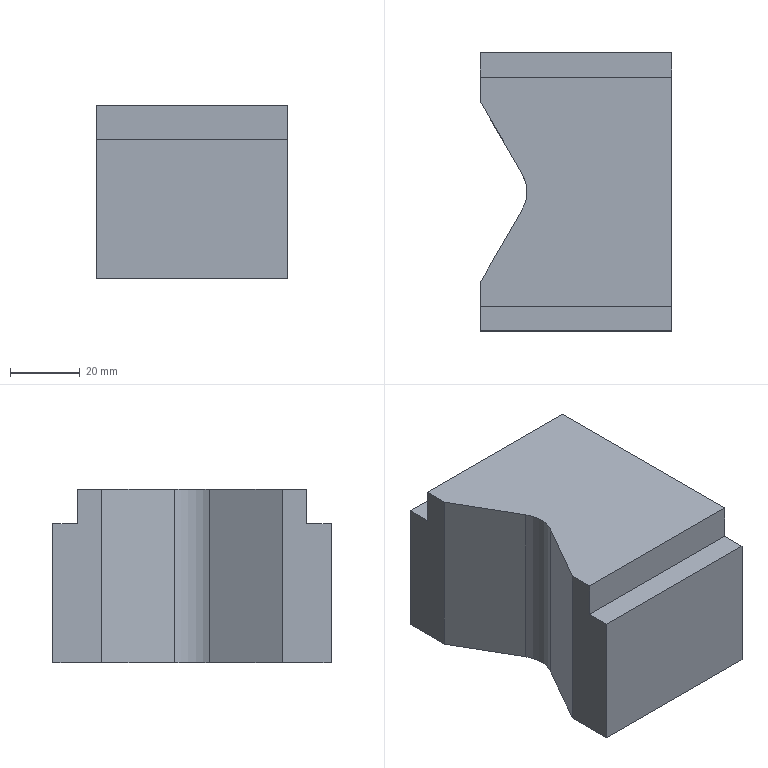Part | STEP file | 001-004-Feeding mechanism push block | 1 solid | 14 faces | box 55 x 80 x 50 mm | volume 193083 mm3 | plane 13 | cylinder 1 | commonest cylinder face diameters 20 x1
STEP:
#1=CARTESIAN_POINT('',(0.,0.,0.));
#2=DIRECTION('',(0.,0.,1.));
#3=DIRECTION('',(1.,0.,0.));
#4=AXIS2_PLACEMENT_3D('',#1,#2,#3);
#5=CARTESIAN_POINT('',(-27.5,33.,50.));
#6=VERTEX_POINT('',#5);
#7=CARTESIAN_POINT('',(-27.5,33.,40.));
#8=VERTEX_POINT('',#7);
#9=CARTESIAN_POINT('',(-27.5,33.,50.));
#10=DIRECTION('',(0.,0.,-1.));
#11=VECTOR('',#10,1.);
#12=LINE('',#9,#11);
#13=CARTESIAN_POINT('',(-27.5,-40.,50.));
#14=DIRECTION('',(1.,0.,0.));
#15=DIRECTION('',(0.,0.,-1.));
#16=AXIS2_PLACEMENT_3D('',#13,#14,#15);
#17=PLANE('',#16);
#18=CARTESIAN_POINT('',(0.,73.));
#19=DIRECTION('',(1.,0.));
#20=VECTOR('',#19,1.);
#21=LINE('',#18,#20);
#22=(GEOMETRIC_REPRESENTATION_CONTEXT(2)PARAMETRIC_REPRESENTATION_CONTEXT()REPRESENTATION_CONTEXT('',''));
#23=DEFINITIONAL_REPRESENTATION('',(#21),#22);
#24=PCURVE('',#17,#23);
#25=CARTESIAN_POINT('',(-27.5,33.,50.));
#26=DIRECTION('',(0.,-1.,0.));
#27=DIRECTION('',(0.,0.,-1.));
#28=AXIS2_PLACEMENT_3D('',#25,#26,#27);
#29=PLANE('',#28);
#30=CARTESIAN_POINT('',(0.,0.));
#31=DIRECTION('',(1.,0.));
#32=VECTOR('',#31,1.);
#33=LINE('',#30,#32);
#34=(GEOMETRIC_REPRESENTATION_CONTEXT(2)PARAMETRIC_REPRESENTATION_CONTEXT()REPRESENTATION_CONTEXT('',''));
#35=DEFINITIONAL_REPRESENTATION('',(#33),#34);
#36=PCURVE('',#29,#35);
#37=SURFACE_CURVE('',#12,(#24,#36),.PCURVE_S1.);
#38=EDGE_CURVE('',#6,#8,#37,.T.);
#39=ORIENTED_EDGE('',*,*,#38,.T.);
#40=CARTESIAN_POINT('',(-27.5,40.,40.));
#41=VERTEX_POINT('',#40);
#42=CARTESIAN_POINT('',(-27.5,40.,40.));
#43=DIRECTION('',(0.,1.,0.));
#44=VECTOR('',#43,1.);
#45=LINE('',#42,#44);
#46=CARTESIAN_POINT('',(10.,80.));
#47=DIRECTION('',(0.,1.));
#48=VECTOR('',#47,1.);
#49=LINE('',#46,#48);
#50=(GEOMETRIC_REPRESENTATION_CONTEXT(2)PARAMETRIC_REPRESENTATION_CONTEXT()REPRESENTATION_CONTEXT('',''));
#51=DEFINITIONAL_REPRESENTATION('',(#49),#50);
#52=PCURVE('',#17,#51);
#53=CARTESIAN_POINT('',(-27.5,40.,40.));
#54=DIRECTION('',(0.,0.,-1.));
#55=DIRECTION('',(-1.,0.,0.));
#56=AXIS2_PLACEMENT_3D('',#53,#54,#55);
#57=PLANE('',#56);
#58=CARTESIAN_POINT('',(0.,0.));
#59=DIRECTION('',(0.,1.));
#60=VECTOR('',#59,1.);
#61=LINE('',#58,#60);
#62=(GEOMETRIC_REPRESENTATION_CONTEXT(2)PARAMETRIC_REPRESENTATION_CONTEXT()REPRESENTATION_CONTEXT('',''));
#63=DEFINITIONAL_REPRESENTATION('',(#61),#62);
#64=PCURVE('',#57,#63);
#65=SURFACE_CURVE('',#45,(#52,#64),.PCURVE_S1.);
#66=EDGE_CURVE('',#8,#41,#65,.T.);
#67=ORIENTED_EDGE('',*,*,#66,.T.);
#68=CARTESIAN_POINT('',(-27.5,40.,0.));
#69=VERTEX_POINT('',#68);
#70=CARTESIAN_POINT('',(-27.5,40.,50.));
#71=DIRECTION('',(0.,0.,-1.));
#72=VECTOR('',#71,1.);
#73=LINE('',#70,#72);
#74=CARTESIAN_POINT('',(0.,80.));
#75=DIRECTION('',(1.,0.));
#76=VECTOR('',#75,1.);
#77=LINE('',#74,#76);
#78=(GEOMETRIC_REPRESENTATION_CONTEXT(2)PARAMETRIC_REPRESENTATION_CONTEXT()REPRESENTATION_CONTEXT('',''));
#79=DEFINITIONAL_REPRESENTATION('',(#77),#78);
#80=PCURVE('',#17,#79);
#81=CARTESIAN_POINT('',(-27.5,40.,50.));
#82=DIRECTION('',(0.,-1.,0.));
#83=DIRECTION('',(0.,0.,-1.));
#84=AXIS2_PLACEMENT_3D('',#81,#82,#83);
#85=PLANE('',#84);
#86=CARTESIAN_POINT('',(0.,0.));
#87=DIRECTION('',(1.,0.));
#88=VECTOR('',#87,1.);
#89=LINE('',#86,#88);
#90=(GEOMETRIC_REPRESENTATION_CONTEXT(2)PARAMETRIC_REPRESENTATION_CONTEXT()REPRESENTATION_CONTEXT('',''));
#91=DEFINITIONAL_REPRESENTATION('',(#89),#90);
#92=PCURVE('',#85,#91);
#93=SURFACE_CURVE('',#73,(#80,#92),.PCURVE_S1.);
#94=EDGE_CURVE('',#41,#69,#93,.T.);
#95=ORIENTED_EDGE('',*,*,#94,.T.);
#96=CARTESIAN_POINT('',(-27.5,25.981,0.));
#97=VERTEX_POINT('',#96);
#98=CARTESIAN_POINT('',(-27.5,-40.,0.));
#99=DIRECTION('',(0.,-1.,0.));
#100=VECTOR('',#99,1.);
#101=LINE('',#98,#100);
#102=CARTESIAN_POINT('',(50.,0.));
#103=DIRECTION('',(0.,-1.));
#104=VECTOR('',#103,1.);
#105=LINE('',#102,#104);
#106=(GEOMETRIC_REPRESENTATION_CONTEXT(2)PARAMETRIC_REPRESENTATION_CONTEXT()REPRESENTATION_CONTEXT('',''));
#107=DEFINITIONAL_REPRESENTATION('',(#105),#106);
#108=PCURVE('',#17,#107);
#109=CARTESIAN_POINT('',(0.,0.,0.));
#110=DIRECTION('',(0.,0.,-1.));
#111=DIRECTION('',(-1.,0.,0.));
#112=AXIS2_PLACEMENT_3D('',#109,#110,#111);
#113=PLANE('',#112);
#114=CARTESIAN_POINT('',(27.5,-40.));
#115=DIRECTION('',(0.,-1.));
#116=VECTOR('',#115,1.);
#117=LINE('',#114,#116);
#118=(GEOMETRIC_REPRESENTATION_CONTEXT(2)PARAMETRIC_REPRESENTATION_CONTEXT()REPRESENTATION_CONTEXT('',''));
#119=DEFINITIONAL_REPRESENTATION('',(#117),#118);
#120=PCURVE('',#113,#119);
#121=SURFACE_CURVE('',#101,(#108,#120),.PCURVE_S1.);
#122=EDGE_CURVE('',#69,#97,#121,.T.);
#123=ORIENTED_EDGE('',*,*,#122,.T.);
#124=CARTESIAN_POINT('',(-27.5,25.981,50.));
#125=VERTEX_POINT('',#124);
#126=CARTESIAN_POINT('',(-27.5,25.981,0.));
#127=DIRECTION('',(0.,0.,1.));
#128=VECTOR('',#127,1.);
#129=LINE('',#126,#128);
#130=CARTESIAN_POINT('',(50.,65.981));
#131=DIRECTION('',(-1.,0.));
#132=VECTOR('',#131,1.);
#133=LINE('',#130,#132);
#134=(GEOMETRIC_REPRESENTATION_CONTEXT(2)PARAMETRIC_REPRESENTATION_CONTEXT()REPRESENTATION_CONTEXT('',''));
#135=DEFINITIONAL_REPRESENTATION('',(#133),#134);
#136=PCURVE('',#17,#135);
#137=CARTESIAN_POINT('',(-27.5,25.981,0.));
#138=DIRECTION('',(0.866,0.5,0.));
#139=DIRECTION('',(-0.5,0.866,0.));
#140=AXIS2_PLACEMENT_3D('',#137,#138,#139);
#141=PLANE('',#140);
#142=CARTESIAN_POINT('',(0.,0.));
#143=DIRECTION('',(0.,1.));
#144=VECTOR('',#143,1.);
#145=LINE('',#142,#144);
#146=(GEOMETRIC_REPRESENTATION_CONTEXT(2)PARAMETRIC_REPRESENTATION_CONTEXT()REPRESENTATION_CONTEXT('',''));
#147=DEFINITIONAL_REPRESENTATION('',(#145),#146);
#148=PCURVE('',#141,#147);
#149=SURFACE_CURVE('',#129,(#136,#148),.PCURVE_S1.);
#150=EDGE_CURVE('',#97,#125,#149,.T.);
#151=ORIENTED_EDGE('',*,*,#150,.T.);
#152=CARTESIAN_POINT('',(-27.5,-40.,50.));
#153=DIRECTION('',(0.,-1.,0.));
#154=VECTOR('',#153,1.);
#155=LINE('',#152,#154);
#156=CARTESIAN_POINT('',(0.,0.));
#157=DIRECTION('',(0.,-1.));
#158=VECTOR('',#157,1.);
#159=LINE('',#156,#158);
#160=(GEOMETRIC_REPRESENTATION_CONTEXT(2)PARAMETRIC_REPRESENTATION_CONTEXT()REPRESENTATION_CONTEXT('',''));
#161=DEFINITIONAL_REPRESENTATION('',(#159),#160);
#162=PCURVE('',#17,#161);
#163=CARTESIAN_POINT('',(0.,0.,50.));
#164=DIRECTION('',(0.,0.,-1.));
#165=DIRECTION('',(-1.,0.,0.));
#166=AXIS2_PLACEMENT_3D('',#163,#164,#165);
#167=PLANE('',#166);
#168=CARTESIAN_POINT('',(27.5,-40.));
#169=DIRECTION('',(0.,-1.));
#170=VECTOR('',#169,1.);
#171=LINE('',#168,#170);
#172=(GEOMETRIC_REPRESENTATION_CONTEXT(2)PARAMETRIC_REPRESENTATION_CONTEXT()REPRESENTATION_CONTEXT('',''));
#173=DEFINITIONAL_REPRESENTATION('',(#171),#172);
#174=PCURVE('',#167,#173);
#175=SURFACE_CURVE('',#155,(#162,#174),.PCURVE_S1.);
#176=EDGE_CURVE('',#6,#125,#175,.T.);
#177=ORIENTED_EDGE('',*,*,#176,.F.);
#178=EDGE_LOOP('',(#39,#67,#95,#123,#151,#177));
#179=FACE_BOUND('',#178,.T.);
#180=ADVANCED_FACE('',(#179),#17,.F.);
#181=CARTESIAN_POINT('',(27.5,40.,40.));
#182=VERTEX_POINT('',#181);
#183=CARTESIAN_POINT('',(27.5,40.,0.));
#184=VERTEX_POINT('',#183);
#185=CARTESIAN_POINT('',(27.5,40.,50.));
#186=DIRECTION('',(0.,0.,-1.));
#187=VECTOR('',#186,1.);
#188=LINE('',#185,#187);
#189=CARTESIAN_POINT('',(27.5,-40.,50.));
#190=DIRECTION('',(-1.,0.,0.));
#191=DIRECTION('',(0.,0.,1.));
#192=AXIS2_PLACEMENT_3D('',#189,#190,#191);
#193=PLANE('',#192);
#194=CARTESIAN_POINT('',(0.,80.));
#195=DIRECTION('',(-1.,0.));
#196=VECTOR('',#195,1.);
#197=LINE('',#194,#196);
#198=(GEOMETRIC_REPRESENTATION_CONTEXT(2)PARAMETRIC_REPRESENTATION_CONTEXT()REPRESENTATION_CONTEXT('',''));
#199=DEFINITIONAL_REPRESENTATION('',(#197),#198);
#200=PCURVE('',#193,#199);
#201=CARTESIAN_POINT('',(0.,55.));
#202=DIRECTION('',(1.,0.));
#203=VECTOR('',#202,1.);
#204=LINE('',#201,#203);
#205=(GEOMETRIC_REPRESENTATION_CONTEXT(2)PARAMETRIC_REPRESENTATION_CONTEXT()REPRESENTATION_CONTEXT('',''));
#206=DEFINITIONAL_REPRESENTATION('',(#204),#205);
#207=PCURVE('',#85,#206);
#208=SURFACE_CURVE('',#188,(#200,#207),.PCURVE_S1.);
#209=EDGE_CURVE('',#182,#184,#208,.T.);
#210=ORIENTED_EDGE('',*,*,#209,.F.);
#211=CARTESIAN_POINT('',(27.5,33.,40.));
#212=VERTEX_POINT('',#211);
#213=CARTESIAN_POINT('',(27.5,40.,40.));
#214=DIRECTION('',(0.,1.,0.));
#215=VECTOR('',#214,1.);
#216=LINE('',#213,#215);
#217=CARTESIAN_POINT('',(-10.,80.));
#218=DIRECTION('',(0.,1.));
#219=VECTOR('',#218,1.);
#220=LINE('',#217,#219);
#221=(GEOMETRIC_REPRESENTATION_CONTEXT(2)PARAMETRIC_REPRESENTATION_CONTEXT()REPRESENTATION_CONTEXT('',''));
#222=DEFINITIONAL_REPRESENTATION('',(#220),#221);
#223=PCURVE('',#193,#222);
#224=CARTESIAN_POINT('',(-55.,0.));
#225=DIRECTION('',(0.,1.));
#226=VECTOR('',#225,1.);
#227=LINE('',#224,#226);
#228=(GEOMETRIC_REPRESENTATION_CONTEXT(2)PARAMETRIC_REPRESENTATION_CONTEXT()REPRESENTATION_CONTEXT('',''));
#229=DEFINITIONAL_REPRESENTATION('',(#227),#228);
#230=PCURVE('',#57,#229);
#231=SURFACE_CURVE('',#216,(#223,#230),.PCURVE_S1.);
#232=EDGE_CURVE('',#212,#182,#231,.T.);
#233=ORIENTED_EDGE('',*,*,#232,.F.);
#234=CARTESIAN_POINT('',(27.5,33.,50.));
#235=VERTEX_POINT('',#234);
#236=CARTESIAN_POINT('',(27.5,33.,50.));
#237=DIRECTION('',(0.,0.,-1.));
#238=VECTOR('',#237,1.);
#239=LINE('',#236,#238);
#240=CARTESIAN_POINT('',(0.,73.));
#241=DIRECTION('',(-1.,0.));
#242=VECTOR('',#241,1.);
#243=LINE('',#240,#242);
#244=(GEOMETRIC_REPRESENTATION_CONTEXT(2)PARAMETRIC_REPRESENTATION_CONTEXT()REPRESENTATION_CONTEXT('',''));
#245=DEFINITIONAL_REPRESENTATION('',(#243),#244);
#246=PCURVE('',#193,#245);
#247=CARTESIAN_POINT('',(0.,55.));
#248=DIRECTION('',(1.,0.));
#249=VECTOR('',#248,1.);
#250=LINE('',#247,#249);
#251=(GEOMETRIC_REPRESENTATION_CONTEXT(2)PARAMETRIC_REPRESENTATION_CONTEXT()REPRESENTATION_CONTEXT('',''));
#252=DEFINITIONAL_REPRESENTATION('',(#250),#251);
#253=PCURVE('',#29,#252);
#254=SURFACE_CURVE('',#239,(#246,#253),.PCURVE_S1.);
#255=EDGE_CURVE('',#235,#212,#254,.T.);
#256=ORIENTED_EDGE('',*,*,#255,.F.);
#257=CARTESIAN_POINT('',(27.5,-33.,50.));
#258=VERTEX_POINT('',#257);
#259=CARTESIAN_POINT('',(27.5,-40.,50.));
#260=DIRECTION('',(0.,1.,0.));
#261=VECTOR('',#260,1.);
#262=LINE('',#259,#261);
#263=CARTESIAN_POINT('',(0.,0.));
#264=DIRECTION('',(0.,1.));
#265=VECTOR('',#264,1.);
#266=LINE('',#263,#265);
#267=(GEOMETRIC_REPRESENTATION_CONTEXT(2)PARAMETRIC_REPRESENTATION_CONTEXT()REPRESENTATION_CONTEXT('',''));
#268=DEFINITIONAL_REPRESENTATION('',(#266),#267);
#269=PCURVE('',#193,#268);
#270=CARTESIAN_POINT('',(-27.5,-40.));
#271=DIRECTION('',(0.,1.));
#272=VECTOR('',#271,1.);
#273=LINE('',#270,#272);
#274=(GEOMETRIC_REPRESENTATION_CONTEXT(2)PARAMETRIC_REPRESENTATION_CONTEXT()REPRESENTATION_CONTEXT('',''));
#275=DEFINITIONAL_REPRESENTATION('',(#273),#274);
#276=PCURVE('',#167,#275);
#277=SURFACE_CURVE('',#262,(#269,#276),.PCURVE_S1.);
#278=EDGE_CURVE('',#258,#235,#277,.T.);
#279=ORIENTED_EDGE('',*,*,#278,.F.);
#280=CARTESIAN_POINT('',(27.5,-33.,40.));
#281=VERTEX_POINT('',#280);
#282=CARTESIAN_POINT('',(27.5,-33.,50.));
#283=DIRECTION('',(0.,0.,1.));
#284=VECTOR('',#283,1.);
#285=LINE('',#282,#284);
#286=CARTESIAN_POINT('',(0.,7.));
#287=DIRECTION('',(1.,0.));
#288=VECTOR('',#287,1.);
#289=LINE('',#286,#288);
#290=(GEOMETRIC_REPRESENTATION_CONTEXT(2)PARAMETRIC_REPRESENTATION_CONTEXT()REPRESENTATION_CONTEXT('',''));
#291=DEFINITIONAL_REPRESENTATION('',(#289),#290);
#292=PCURVE('',#193,#291);
#293=CARTESIAN_POINT('',(-27.5,-33.,50.));
#294=DIRECTION('',(0.,1.,0.));
#295=DIRECTION('',(0.,0.,1.));
#296=AXIS2_PLACEMENT_3D('',#293,#294,#295);
#297=PLANE('',#296);
#298=CARTESIAN_POINT('',(0.,55.));
#299=DIRECTION('',(1.,0.));
#300=VECTOR('',#299,1.);
#301=LINE('',#298,#300);
#302=(GEOMETRIC_REPRESENTATION_CONTEXT(2)PARAMETRIC_REPRESENTATION_CONTEXT()REPRESENTATION_CONTEXT('',''));
#303=DEFINITIONAL_REPRESENTATION('',(#301),#302);
#304=PCURVE('',#297,#303);
#305=SURFACE_CURVE('',#285,(#292,#304),.PCURVE_S1.);
#306=EDGE_CURVE('',#281,#258,#305,.T.);
#307=ORIENTED_EDGE('',*,*,#306,.F.);
#308=CARTESIAN_POINT('',(27.5,-40.,40.));
#309=VERTEX_POINT('',#308);
#310=CARTESIAN_POINT('',(27.5,-40.,40.));
#311=DIRECTION('',(0.,1.,0.));
#312=VECTOR('',#311,1.);
#313=LINE('',#310,#312);
#314=CARTESIAN_POINT('',(-10.,0.));
#315=DIRECTION('',(0.,1.));
#316=VECTOR('',#315,1.);
#317=LINE('',#314,#316);
#318=(GEOMETRIC_REPRESENTATION_CONTEXT(2)PARAMETRIC_REPRESENTATION_CONTEXT()REPRESENTATION_CONTEXT('',''));
#319=DEFINITIONAL_REPRESENTATION('',(#317),#318);
#320=PCURVE('',#193,#319);
#321=CARTESIAN_POINT('',(-27.5,-40.,40.));
#322=DIRECTION('',(0.,0.,-1.));
#323=DIRECTION('',(-1.,0.,0.));
#324=AXIS2_PLACEMENT_3D('',#321,#322,#323);
#325=PLANE('',#324);
#326=CARTESIAN_POINT('',(-55.,0.));
#327=DIRECTION('',(0.,1.));
#328=VECTOR('',#327,1.);
#329=LINE('',#326,#328);
#330=(GEOMETRIC_REPRESENTATION_CONTEXT(2)PARAMETRIC_REPRESENTATION_CONTEXT()REPRESENTATION_CONTEXT('',''));
#331=DEFINITIONAL_REPRESENTATION('',(#329),#330);
#332=PCURVE('',#325,#331);
#333=SURFACE_CURVE('',#313,(#320,#332),.PCURVE_S1.);
#334=EDGE_CURVE('',#309,#281,#333,.T.);
#335=ORIENTED_EDGE('',*,*,#334,.F.);
#336=CARTESIAN_POINT('',(27.5,-40.,0.));
#337=VERTEX_POINT('',#336);
#338=CARTESIAN_POINT('',(27.5,-40.,50.));
#339=DIRECTION('',(0.,0.,-1.));
#340=VECTOR('',#339,1.);
#341=LINE('',#338,#340);
#342=CARTESIAN_POINT('',(0.,0.));
#343=DIRECTION('',(-1.,0.));
#344=VECTOR('',#343,1.);
#345=LINE('',#342,#344);
#346=(GEOMETRIC_REPRESENTATION_CONTEXT(2)PARAMETRIC_REPRESENTATION_CONTEXT()REPRESENTATION_CONTEXT('',''));
#347=DEFINITIONAL_REPRESENTATION('',(#345),#346);
#348=PCURVE('',#193,#347);
#349=CARTESIAN_POINT('',(-27.5,-40.,50.));
#350=DIRECTION('',(0.,1.,0.));
#351=DIRECTION('',(0.,0.,1.));
#352=AXIS2_PLACEMENT_3D('',#349,#350,#351);
#353=PLANE('',#352);
#354=CARTESIAN_POINT('',(0.,55.));
#355=DIRECTION('',(-1.,0.));
#356=VECTOR('',#355,1.);
#357=LINE('',#354,#356);
#358=(GEOMETRIC_REPRESENTATION_CONTEXT(2)PARAMETRIC_REPRESENTATION_CONTEXT()REPRESENTATION_CONTEXT('',''));
#359=DEFINITIONAL_REPRESENTATION('',(#357),#358);
#360=PCURVE('',#353,#359);
#361=SURFACE_CURVE('',#341,(#348,#360),.PCURVE_S1.);
#362=EDGE_CURVE('',#309,#337,#361,.T.);
#363=ORIENTED_EDGE('',*,*,#362,.T.);
#364=CARTESIAN_POINT('',(27.5,-40.,0.));
#365=DIRECTION('',(0.,1.,0.));
#366=VECTOR('',#365,1.);
#367=LINE('',#364,#366);
#368=CARTESIAN_POINT('',(-50.,0.));
#369=DIRECTION('',(0.,1.));
#370=VECTOR('',#369,1.);
#371=LINE('',#368,#370);
#372=(GEOMETRIC_REPRESENTATION_CONTEXT(2)PARAMETRIC_REPRESENTATION_CONTEXT()REPRESENTATION_CONTEXT('',''));
#373=DEFINITIONAL_REPRESENTATION('',(#371),#372);
#374=PCURVE('',#193,#373);
#375=CARTESIAN_POINT('',(-27.5,-40.));
#376=DIRECTION('',(0.,1.));
#377=VECTOR('',#376,1.);
#378=LINE('',#375,#377);
#379=(GEOMETRIC_REPRESENTATION_CONTEXT(2)PARAMETRIC_REPRESENTATION_CONTEXT()REPRESENTATION_CONTEXT('',''));
#380=DEFINITIONAL_REPRESENTATION('',(#378),#379);
#381=PCURVE('',#113,#380);
#382=SURFACE_CURVE('',#367,(#374,#381),.PCURVE_S1.);
#383=EDGE_CURVE('',#337,#184,#382,.T.);
#384=ORIENTED_EDGE('',*,*,#383,.T.);
#385=EDGE_LOOP('',(#210,#233,#256,#279,#307,#335,#363,#384));
#386=FACE_BOUND('',#385,.T.);
#387=ADVANCED_FACE('',(#386),#193,.F.);
#388=ORIENTED_EDGE('',*,*,#94,.F.);
#389=CARTESIAN_POINT('',(-27.5,40.,40.));
#390=DIRECTION('',(1.,0.,0.));
#391=VECTOR('',#390,1.);
#392=LINE('',#389,#391);
#393=CARTESIAN_POINT('',(10.,0.));
#394=DIRECTION('',(0.,1.));
#395=VECTOR('',#394,1.);
#396=LINE('',#393,#395);
#397=(GEOMETRIC_REPRESENTATION_CONTEXT(2)PARAMETRIC_REPRESENTATION_CONTEXT()REPRESENTATION_CONTEXT('',''));
#398=DEFINITIONAL_REPRESENTATION('',(#396),#397);
#399=PCURVE('',#85,#398);
#400=CARTESIAN_POINT('',(0.,0.));
#401=DIRECTION('',(-1.,0.));
#402=VECTOR('',#401,1.);
#403=LINE('',#400,#402);
#404=(GEOMETRIC_REPRESENTATION_CONTEXT(2)PARAMETRIC_REPRESENTATION_CONTEXT()REPRESENTATION_CONTEXT('',''));
#405=DEFINITIONAL_REPRESENTATION('',(#403),#404);
#406=PCURVE('',#57,#405);
#407=SURFACE_CURVE('',#392,(#399,#406),.PCURVE_S1.);
#408=EDGE_CURVE('',#41,#182,#407,.T.);
#409=ORIENTED_EDGE('',*,*,#408,.T.);
#410=ORIENTED_EDGE('',*,*,#209,.T.);
#411=CARTESIAN_POINT('',(-27.5,40.,0.));
#412=DIRECTION('',(-1.,0.,0.));
#413=VECTOR('',#412,1.);
#414=LINE('',#411,#413);
#415=CARTESIAN_POINT('',(50.,0.));
#416=DIRECTION('',(0.,-1.));
#417=VECTOR('',#416,1.);
#418=LINE('',#415,#417);
#419=(GEOMETRIC_REPRESENTATION_CONTEXT(2)PARAMETRIC_REPRESENTATION_CONTEXT()REPRESENTATION_CONTEXT('',''));
#420=DEFINITIONAL_REPRESENTATION('',(#418),#419);
#421=PCURVE('',#85,#420);
#422=CARTESIAN_POINT('',(27.5,40.));
#423=DIRECTION('',(1.,0.));
#424=VECTOR('',#423,1.);
#425=LINE('',#422,#424);
#426=(GEOMETRIC_REPRESENTATION_CONTEXT(2)PARAMETRIC_REPRESENTATION_CONTEXT()REPRESENTATION_CONTEXT('',''));
#427=DEFINITIONAL_REPRESENTATION('',(#425),#426);
#428=PCURVE('',#113,#427);
#429=SURFACE_CURVE('',#414,(#421,#428),.PCURVE_S1.);
#430=EDGE_CURVE('',#184,#69,#429,.T.);
#431=ORIENTED_EDGE('',*,*,#430,.T.);
#432=EDGE_LOOP('',(#388,#409,#410,#431));
#433=FACE_BOUND('',#432,.T.);
#434=ADVANCED_FACE('',(#433),#85,.F.);
#435=CARTESIAN_POINT('',(-27.5,-40.,40.));
#436=VERTEX_POINT('',#435);
#437=CARTESIAN_POINT('',(-27.5,-33.,40.));
#438=VERTEX_POINT('',#437);
#439=CARTESIAN_POINT('',(-27.5,-40.,40.));
#440=DIRECTION('',(0.,1.,0.));
#441=VECTOR('',#440,1.);
#442=LINE('',#439,#441);
#443=CARTESIAN_POINT('',(-27.5,-40.,50.));
#444=DIRECTION('',(1.,0.,0.));
#445=DIRECTION('',(0.,0.,-1.));
#446=AXIS2_PLACEMENT_3D('',#443,#444,#445);
#447=PLANE('',#446);
#448=CARTESIAN_POINT('',(10.,0.));
#449=DIRECTION('',(0.,1.));
#450=VECTOR('',#449,1.);
#451=LINE('',#448,#450);
#452=(GEOMETRIC_REPRESENTATION_CONTEXT(2)PARAMETRIC_REPRESENTATION_CONTEXT()REPRESENTATION_CONTEXT('',''));
#453=DEFINITIONAL_REPRESENTATION('',(#451),#452);
#454=PCURVE('',#447,#453);
#455=CARTESIAN_POINT('',(0.,0.));
#456=DIRECTION('',(0.,1.));
#457=VECTOR('',#456,1.);
#458=LINE('',#455,#457);
#459=(GEOMETRIC_REPRESENTATION_CONTEXT(2)PARAMETRIC_REPRESENTATION_CONTEXT()REPRESENTATION_CONTEXT('',''));
#460=DEFINITIONAL_REPRESENTATION('',(#458),#459);
#461=PCURVE('',#325,#460);
#462=SURFACE_CURVE('',#442,(#454,#461),.PCURVE_S1.);
#463=EDGE_CURVE('',#436,#438,#462,.T.);
#464=ORIENTED_EDGE('',*,*,#463,.T.);
#465=CARTESIAN_POINT('',(-27.5,-33.,50.));
#466=VERTEX_POINT('',#465);
#467=CARTESIAN_POINT('',(-27.5,-33.,50.));
#468=DIRECTION('',(0.,0.,1.));
#469=VECTOR('',#468,1.);
#470=LINE('',#467,#469);
#471=CARTESIAN_POINT('',(0.,7.));
#472=DIRECTION('',(-1.,0.));
#473=VECTOR('',#472,1.);
#474=LINE('',#471,#473);
#475=(GEOMETRIC_REPRESENTATION_CONTEXT(2)PARAMETRIC_REPRESENTATION_CONTEXT()REPRESENTATION_CONTEXT('',''));
#476=DEFINITIONAL_REPRESENTATION('',(#474),#475);
#477=PCURVE('',#447,#476);
#478=CARTESIAN_POINT('',(0.,0.));
#479=DIRECTION('',(1.,0.));
#480=VECTOR('',#479,1.);
#481=LINE('',#478,#480);
#482=(GEOMETRIC_REPRESENTATION_CONTEXT(2)PARAMETRIC_REPRESENTATION_CONTEXT()REPRESENTATION_CONTEXT('',''));
#483=DEFINITIONAL_REPRESENTATION('',(#481),#482);
#484=PCURVE('',#297,#483);
#485=SURFACE_CURVE('',#470,(#477,#484),.PCURVE_S1.);
#486=EDGE_CURVE('',#438,#466,#485,.T.);
#487=ORIENTED_EDGE('',*,*,#486,.T.);
#488=CARTESIAN_POINT('',(-27.5,-25.981,50.));
#489=VERTEX_POINT('',#488);
#490=CARTESIAN_POINT('',(-27.5,-40.,50.));
#491=DIRECTION('',(0.,-1.,0.));
#492=VECTOR('',#491,1.);
#493=LINE('',#490,#492);
#494=CARTESIAN_POINT('',(0.,0.));
#495=DIRECTION('',(0.,-1.));
#496=VECTOR('',#495,1.);
#497=LINE('',#494,#496);
#498=(GEOMETRIC_REPRESENTATION_CONTEXT(2)PARAMETRIC_REPRESENTATION_CONTEXT()REPRESENTATION_CONTEXT('',''));
#499=DEFINITIONAL_REPRESENTATION('',(#497),#498);
#500=PCURVE('',#447,#499);
#501=CARTESIAN_POINT('',(27.5,-40.));
#502=DIRECTION('',(0.,-1.));
#503=VECTOR('',#502,1.);
#504=LINE('',#501,#503);
#505=(GEOMETRIC_REPRESENTATION_CONTEXT(2)PARAMETRIC_REPRESENTATION_CONTEXT()REPRESENTATION_CONTEXT('',''));
#506=DEFINITIONAL_REPRESENTATION('',(#504),#505);
#507=PCURVE('',#167,#506);
#508=SURFACE_CURVE('',#493,(#500,#507),.PCURVE_S1.);
#509=EDGE_CURVE('',#489,#466,#508,.T.);
#510=ORIENTED_EDGE('',*,*,#509,.F.);
#511=CARTESIAN_POINT('',(-27.5,-25.981,0.));
#512=VERTEX_POINT('',#511);
#513=CARTESIAN_POINT('',(-27.5,-25.981,0.));
#514=DIRECTION('',(0.,0.,1.));
#515=VECTOR('',#514,1.);
#516=LINE('',#513,#515);
#517=CARTESIAN_POINT('',(50.,14.019));
#518=DIRECTION('',(-1.,0.));
#519=VECTOR('',#518,1.);
#520=LINE('',#517,#519);
#521=(GEOMETRIC_REPRESENTATION_CONTEXT(2)PARAMETRIC_REPRESENTATION_CONTEXT()REPRESENTATION_CONTEXT('',''));
#522=DEFINITIONAL_REPRESENTATION('',(#520),#521);
#523=PCURVE('',#447,#522);
#524=CARTESIAN_POINT('',(-27.5,-25.981,0.));
#525=DIRECTION('',(0.866,-0.5,0.));
#526=DIRECTION('',(0.5,0.866,0.));
#527=AXIS2_PLACEMENT_3D('',#524,#525,#526);
#528=PLANE('',#527);
#529=CARTESIAN_POINT('',(0.,0.));
#530=DIRECTION('',(0.,1.));
#531=VECTOR('',#530,1.);
#532=LINE('',#529,#531);
#533=(GEOMETRIC_REPRESENTATION_CONTEXT(2)PARAMETRIC_REPRESENTATION_CONTEXT()REPRESENTATION_CONTEXT('',''));
#534=DEFINITIONAL_REPRESENTATION('',(#532),#533);
#535=PCURVE('',#528,#534);
#536=SURFACE_CURVE('',#516,(#523,#535),.PCURVE_S1.);
#537=EDGE_CURVE('',#512,#489,#536,.T.);
#538=ORIENTED_EDGE('',*,*,#537,.F.);
#539=CARTESIAN_POINT('',(-27.5,-40.,0.));
#540=VERTEX_POINT('',#539);
#541=CARTESIAN_POINT('',(-27.5,-40.,0.));
#542=DIRECTION('',(0.,-1.,0.));
#543=VECTOR('',#542,1.);
#544=LINE('',#541,#543);
#545=CARTESIAN_POINT('',(50.,0.));
#546=DIRECTION('',(0.,-1.));
#547=VECTOR('',#546,1.);
#548=LINE('',#545,#547);
#549=(GEOMETRIC_REPRESENTATION_CONTEXT(2)PARAMETRIC_REPRESENTATION_CONTEXT()REPRESENTATION_CONTEXT('',''));
#550=DEFINITIONAL_REPRESENTATION('',(#548),#549);
#551=PCURVE('',#447,#550);
#552=CARTESIAN_POINT('',(27.5,-40.));
#553=DIRECTION('',(0.,-1.));
#554=VECTOR('',#553,1.);
#555=LINE('',#552,#554);
#556=(GEOMETRIC_REPRESENTATION_CONTEXT(2)PARAMETRIC_REPRESENTATION_CONTEXT()REPRESENTATION_CONTEXT('',''));
#557=DEFINITIONAL_REPRESENTATION('',(#555),#556);
#558=PCURVE('',#113,#557);
#559=SURFACE_CURVE('',#544,(#551,#558),.PCURVE_S1.);
#560=EDGE_CURVE('',#512,#540,#559,.T.);
#561=ORIENTED_EDGE('',*,*,#560,.T.);
#562=CARTESIAN_POINT('',(-27.5,-40.,50.));
#563=DIRECTION('',(0.,0.,-1.));
#564=VECTOR('',#563,1.);
#565=LINE('',#562,#564);
#566=CARTESIAN_POINT('',(0.,0.));
#567=DIRECTION('',(1.,0.));
#568=VECTOR('',#567,1.);
#569=LINE('',#566,#568);
#570=(GEOMETRIC_REPRESENTATION_CONTEXT(2)PARAMETRIC_REPRESENTATION_CONTEXT()REPRESENTATION_CONTEXT('',''));
#571=DEFINITIONAL_REPRESENTATION('',(#569),#570);
#572=PCURVE('',#447,#571);
#573=CARTESIAN_POINT('',(0.,0.));
#574=DIRECTION('',(-1.,0.));
#575=VECTOR('',#574,1.);
#576=LINE('',#573,#575);
#577=(GEOMETRIC_REPRESENTATION_CONTEXT(2)PARAMETRIC_REPRESENTATION_CONTEXT()REPRESENTATION_CONTEXT('',''));
#578=DEFINITIONAL_REPRESENTATION('',(#576),#577);
#579=PCURVE('',#353,#578);
#580=SURFACE_CURVE('',#565,(#572,#579),.PCURVE_S1.);
#581=EDGE_CURVE('',#436,#540,#580,.T.);
#582=ORIENTED_EDGE('',*,*,#581,.F.);
#583=EDGE_LOOP('',(#464,#487,#510,#538,#561,#582));
#584=FACE_BOUND('',#583,.T.);
#585=ADVANCED_FACE('',(#584),#447,.F.);
#586=ORIENTED_EDGE('',*,*,#362,.F.);
#587=CARTESIAN_POINT('',(-27.5,-40.,40.));
#588=DIRECTION('',(1.,0.,0.));
#589=VECTOR('',#588,1.);
#590=LINE('',#587,#589);
#591=CARTESIAN_POINT('',(-10.,0.));
#592=DIRECTION('',(0.,1.));
#593=VECTOR('',#592,1.);
#594=LINE('',#591,#593);
#595=(GEOMETRIC_REPRESENTATION_CONTEXT(2)PARAMETRIC_REPRESENTATION_CONTEXT()REPRESENTATION_CONTEXT('',''));
#596=DEFINITIONAL_REPRESENTATION('',(#594),#595);
#597=PCURVE('',#353,#596);
#598=CARTESIAN_POINT('',(0.,0.));
#599=DIRECTION('',(-1.,0.));
#600=VECTOR('',#599,1.);
#601=LINE('',#598,#600);
#602=(GEOMETRIC_REPRESENTATION_CONTEXT(2)PARAMETRIC_REPRESENTATION_CONTEXT()REPRESENTATION_CONTEXT('',''));
#603=DEFINITIONAL_REPRESENTATION('',(#601),#602);
#604=PCURVE('',#325,#603);
#605=SURFACE_CURVE('',#590,(#597,#604),.PCURVE_S1.);
#606=EDGE_CURVE('',#436,#309,#605,.T.);
#607=ORIENTED_EDGE('',*,*,#606,.F.);
#608=ORIENTED_EDGE('',*,*,#581,.T.);
#609=CARTESIAN_POINT('',(-27.5,-40.,0.));
#610=DIRECTION('',(1.,0.,0.));
#611=VECTOR('',#610,1.);
#612=LINE('',#609,#611);
#613=CARTESIAN_POINT('',(-50.,0.));
#614=DIRECTION('',(0.,1.));
#615=VECTOR('',#614,1.);
#616=LINE('',#613,#615);
#617=(GEOMETRIC_REPRESENTATION_CONTEXT(2)PARAMETRIC_REPRESENTATION_CONTEXT()REPRESENTATION_CONTEXT('',''));
#618=DEFINITIONAL_REPRESENTATION('',(#616),#617);
#619=PCURVE('',#353,#618);
#620=CARTESIAN_POINT('',(27.5,-40.));
#621=DIRECTION('',(-1.,0.));
#622=VECTOR('',#621,1.);
#623=LINE('',#620,#622);
#624=(GEOMETRIC_REPRESENTATION_CONTEXT(2)PARAMETRIC_REPRESENTATION_CONTEXT()REPRESENTATION_CONTEXT('',''));
#625=DEFINITIONAL_REPRESENTATION('',(#623),#624);
#626=PCURVE('',#113,#625);
#627=SURFACE_CURVE('',#612,(#619,#626),.PCURVE_S1.);
#628=EDGE_CURVE('',#540,#337,#627,.T.);
#629=ORIENTED_EDGE('',*,*,#628,.T.);
#630=EDGE_LOOP('',(#586,#607,#608,#629));
#631=FACE_BOUND('',#630,.T.);
#632=ADVANCED_FACE('',(#631),#353,.F.);
#633=ORIENTED_EDGE('',*,*,#278,.T.);
#634=CARTESIAN_POINT('',(-27.5,33.,50.));
#635=DIRECTION('',(1.,0.,0.));
#636=VECTOR('',#635,1.);
#637=LINE('',#634,#636);
#638=CARTESIAN_POINT('',(27.5,33.));
#639=DIRECTION('',(-1.,0.));
#640=VECTOR('',#639,1.);
#641=LINE('',#638,#640);
#642=(GEOMETRIC_REPRESENTATION_CONTEXT(2)PARAMETRIC_REPRESENTATION_CONTEXT()REPRESENTATION_CONTEXT('',''));
#643=DEFINITIONAL_REPRESENTATION('',(#641),#642);
#644=PCURVE('',#167,#643);
#645=CARTESIAN_POINT('',(0.,0.));
#646=DIRECTION('',(0.,1.));
#647=VECTOR('',#646,1.);
#648=LINE('',#645,#647);
#649=(GEOMETRIC_REPRESENTATION_CONTEXT(2)PARAMETRIC_REPRESENTATION_CONTEXT()REPRESENTATION_CONTEXT('',''));
#650=DEFINITIONAL_REPRESENTATION('',(#648),#649);
#651=PCURVE('',#29,#650);
#652=SURFACE_CURVE('',#637,(#644,#651),.PCURVE_S1.);
#653=EDGE_CURVE('',#6,#235,#652,.T.);
#654=ORIENTED_EDGE('',*,*,#653,.F.);
#655=ORIENTED_EDGE('',*,*,#176,.T.);
#656=CARTESIAN_POINT('',(-15.387,5.,50.));
#657=VERTEX_POINT('',#656);
#658=CARTESIAN_POINT('',(-27.5,25.981,50.));
#659=DIRECTION('',(-0.5,0.866,0.));
#660=VECTOR('',#659,1.);
#661=LINE('',#658,#660);
#662=CARTESIAN_POINT('',(27.5,25.981));
#663=DIRECTION('',(0.5,0.866));
#664=VECTOR('',#663,1.);
#665=LINE('',#662,#664);
#666=(GEOMETRIC_REPRESENTATION_CONTEXT(2)PARAMETRIC_REPRESENTATION_CONTEXT()REPRESENTATION_CONTEXT('',''));
#667=DEFINITIONAL_REPRESENTATION('',(#665),#666);
#668=PCURVE('',#167,#667);
#669=CARTESIAN_POINT('',(0.,50.));
#670=DIRECTION('',(1.,0.));
#671=VECTOR('',#670,1.);
#672=LINE('',#669,#671);
#673=(GEOMETRIC_REPRESENTATION_CONTEXT(2)PARAMETRIC_REPRESENTATION_CONTEXT()REPRESENTATION_CONTEXT('',''));
#674=DEFINITIONAL_REPRESENTATION('',(#672),#673);
#675=PCURVE('',#141,#674);
#676=SURFACE_CURVE('',#661,(#668,#675),.PCURVE_S1.);
#677=EDGE_CURVE('',#657,#125,#676,.T.);
#678=ORIENTED_EDGE('',*,*,#677,.F.);
#679=CARTESIAN_POINT('',(-15.387,-5.,50.));
#680=VERTEX_POINT('',#679);
#681=CARTESIAN_POINT('',(-24.047,0.,50.));
#682=DIRECTION('',(0.,0.,-1.));
#683=DIRECTION('',(-1.,0.,0.));
#684=AXIS2_PLACEMENT_3D('',#681,#682,#683);
#685=CIRCLE('',#684,10.);
#686=CARTESIAN_POINT('',(24.047,0.));
#687=DIRECTION('',(1.,0.));
#688=AXIS2_PLACEMENT_2D('',#686,#687);
#689=CIRCLE('',#688,10.);
#690=(GEOMETRIC_REPRESENTATION_CONTEXT(2)PARAMETRIC_REPRESENTATION_CONTEXT()REPRESENTATION_CONTEXT('',''));
#691=DEFINITIONAL_REPRESENTATION('',(#689),#690);
#692=PCURVE('',#167,#691);
#693=CARTESIAN_POINT('',(-24.047,0.,0.));
#694=DIRECTION('',(0.,0.,-1.));
#695=DIRECTION('',(-1.,0.,0.));
#696=AXIS2_PLACEMENT_3D('',#693,#694,#695);
#697=CYLINDRICAL_SURFACE('',#696,10.);
#698=CARTESIAN_POINT('',(0.,-50.));
#699=DIRECTION('',(1.,0.));
#700=VECTOR('',#699,1.);
#701=LINE('',#698,#700);
#702=(GEOMETRIC_REPRESENTATION_CONTEXT(2)PARAMETRIC_REPRESENTATION_CONTEXT()REPRESENTATION_CONTEXT('',''));
#703=DEFINITIONAL_REPRESENTATION('',(#701),#702);
#704=PCURVE('',#697,#703);
#705=SURFACE_CURVE('',#685,(#692,#704),.PCURVE_S1.);
#706=EDGE_CURVE('',#657,#680,#705,.T.);
#707=ORIENTED_EDGE('',*,*,#706,.T.);
#708=CARTESIAN_POINT('',(-27.5,-25.981,50.));
#709=DIRECTION('',(0.5,0.866,0.));
#710=VECTOR('',#709,1.);
#711=LINE('',#708,#710);
#712=CARTESIAN_POINT('',(27.5,-25.981));
#713=DIRECTION('',(-0.5,0.866));
#714=VECTOR('',#713,1.);
#715=LINE('',#712,#714);
#716=(GEOMETRIC_REPRESENTATION_CONTEXT(2)PARAMETRIC_REPRESENTATION_CONTEXT()REPRESENTATION_CONTEXT('',''));
#717=DEFINITIONAL_REPRESENTATION('',(#715),#716);
#718=PCURVE('',#167,#717);
#719=CARTESIAN_POINT('',(0.,50.));
#720=DIRECTION('',(1.,0.));
#721=VECTOR('',#720,1.);
#722=LINE('',#719,#721);
#723=(GEOMETRIC_REPRESENTATION_CONTEXT(2)PARAMETRIC_REPRESENTATION_CONTEXT()REPRESENTATION_CONTEXT('',''));
#724=DEFINITIONAL_REPRESENTATION('',(#722),#723);
#725=PCURVE('',#528,#724);
#726=SURFACE_CURVE('',#711,(#718,#725),.PCURVE_S1.);
#727=EDGE_CURVE('',#489,#680,#726,.T.);
#728=ORIENTED_EDGE('',*,*,#727,.F.);
#729=ORIENTED_EDGE('',*,*,#509,.T.);
#730=CARTESIAN_POINT('',(-27.5,-33.,50.));
#731=DIRECTION('',(1.,0.,0.));
#732=VECTOR('',#731,1.);
#733=LINE('',#730,#732);
#734=CARTESIAN_POINT('',(27.5,-33.));
#735=DIRECTION('',(-1.,0.));
#736=VECTOR('',#735,1.);
#737=LINE('',#734,#736);
#738=(GEOMETRIC_REPRESENTATION_CONTEXT(2)PARAMETRIC_REPRESENTATION_CONTEXT()REPRESENTATION_CONTEXT('',''));
#739=DEFINITIONAL_REPRESENTATION('',(#737),#738);
#740=PCURVE('',#167,#739);
#741=CARTESIAN_POINT('',(0.,0.));
#742=DIRECTION('',(0.,1.));
#743=VECTOR('',#742,1.);
#744=LINE('',#741,#743);
#745=(GEOMETRIC_REPRESENTATION_CONTEXT(2)PARAMETRIC_REPRESENTATION_CONTEXT()REPRESENTATION_CONTEXT('',''));
#746=DEFINITIONAL_REPRESENTATION('',(#744),#745);
#747=PCURVE('',#297,#746);
#748=SURFACE_CURVE('',#733,(#740,#747),.PCURVE_S1.);
#749=EDGE_CURVE('',#466,#258,#748,.T.);
#750=ORIENTED_EDGE('',*,*,#749,.T.);
#751=EDGE_LOOP('',(#633,#654,#655,#678,#707,#728,#729,#750));
#752=FACE_BOUND('',#751,.T.);
#753=ADVANCED_FACE('',(#752),#167,.F.);
#754=CARTESIAN_POINT('',(-15.387,-5.,0.));
#755=VERTEX_POINT('',#754);
#756=CARTESIAN_POINT('',(-27.5,-25.981,0.));
#757=DIRECTION('',(0.5,0.866,0.));
#758=VECTOR('',#757,1.);
#759=LINE('',#756,#758);
#760=CARTESIAN_POINT('',(27.5,-25.981));
#761=DIRECTION('',(-0.5,0.866));
#762=VECTOR('',#761,1.);
#763=LINE('',#760,#762);
#764=(GEOMETRIC_REPRESENTATION_CONTEXT(2)PARAMETRIC_REPRESENTATION_CONTEXT()REPRESENTATION_CONTEXT('',''));
#765=DEFINITIONAL_REPRESENTATION('',(#763),#764);
#766=PCURVE('',#113,#765);
#767=CARTESIAN_POINT('',(0.,0.));
#768=DIRECTION('',(1.,0.));
#769=VECTOR('',#768,1.);
#770=LINE('',#767,#769);
#771=(GEOMETRIC_REPRESENTATION_CONTEXT(2)PARAMETRIC_REPRESENTATION_CONTEXT()REPRESENTATION_CONTEXT('',''));
#772=DEFINITIONAL_REPRESENTATION('',(#770),#771);
#773=PCURVE('',#528,#772);
#774=SURFACE_CURVE('',#759,(#766,#773),.PCURVE_S1.);
#775=EDGE_CURVE('',#512,#755,#774,.T.);
#776=ORIENTED_EDGE('',*,*,#775,.T.);
#777=CARTESIAN_POINT('',(-15.387,5.,0.));
#778=VERTEX_POINT('',#777);
#779=CARTESIAN_POINT('',(-24.047,0.,0.));
#780=DIRECTION('',(0.,0.,1.));
#781=DIRECTION('',(-1.,0.,0.));
#782=AXIS2_PLACEMENT_3D('',#779,#780,#781);
#783=CIRCLE('',#782,10.);
#784=CARTESIAN_POINT('',(34.047,0.));
#785=CARTESIAN_POINT('',(34.047,-17.321));
#786=CARTESIAN_POINT('',(19.047,-8.66));
#787=CARTESIAN_POINT('',(4.047,0.));
#788=CARTESIAN_POINT('',(19.047,8.66));
#789=CARTESIAN_POINT('',(34.047,17.321));
#790=CARTESIAN_POINT('',(34.047,0.));
#791=(BOUNDED_CURVE()B_SPLINE_CURVE(2,(#784,#785,#786,#787,#788,#789,#790),.UNSPECIFIED.,.T.,.F.)B_SPLINE_CURVE_WITH_KNOTS((1,2,2,2,2,1),(-2.094,0.,2.094,4.189,6.283,8.378),.UNSPECIFIED.)CURVE()GEOMETRIC_REPRESENTATION_ITEM()RATIONAL_B_SPLINE_CURVE((1.,0.5,1.,0.5,1.,0.5,1.))REPRESENTATION_ITEM(''));
#792=(GEOMETRIC_REPRESENTATION_CONTEXT(2)PARAMETRIC_REPRESENTATION_CONTEXT()REPRESENTATION_CONTEXT('',''));
#793=DEFINITIONAL_REPRESENTATION('',(#791),#792);
#794=PCURVE('',#113,#793);
#795=CARTESIAN_POINT('',(6.283,0.));
#796=DIRECTION('',(-1.,0.));
#797=VECTOR('',#796,1.);
#798=LINE('',#795,#797);
#799=(GEOMETRIC_REPRESENTATION_CONTEXT(2)PARAMETRIC_REPRESENTATION_CONTEXT()REPRESENTATION_CONTEXT('',''));
#800=DEFINITIONAL_REPRESENTATION('',(#798),#799);
#801=PCURVE('',#697,#800);
#802=SURFACE_CURVE('',#783,(#794,#801),.PCURVE_S1.);
#803=EDGE_CURVE('',#755,#778,#802,.T.);
#804=ORIENTED_EDGE('',*,*,#803,.T.);
#805=CARTESIAN_POINT('',(-27.5,25.981,0.));
#806=DIRECTION('',(-0.5,0.866,0.));
#807=VECTOR('',#806,1.);
#808=LINE('',#805,#807);
#809=CARTESIAN_POINT('',(27.5,25.981));
#810=DIRECTION('',(0.5,0.866));
#811=VECTOR('',#810,1.);
#812=LINE('',#809,#811);
#813=(GEOMETRIC_REPRESENTATION_CONTEXT(2)PARAMETRIC_REPRESENTATION_CONTEXT()REPRESENTATION_CONTEXT('',''));
#814=DEFINITIONAL_REPRESENTATION('',(#812),#813);
#815=PCURVE('',#113,#814);
#816=CARTESIAN_POINT('',(0.,0.));
#817=DIRECTION('',(1.,0.));
#818=VECTOR('',#817,1.);
#819=LINE('',#816,#818);
#820=(GEOMETRIC_REPRESENTATION_CONTEXT(2)PARAMETRIC_REPRESENTATION_CONTEXT()REPRESENTATION_CONTEXT('',''));
#821=DEFINITIONAL_REPRESENTATION('',(#819),#820);
#822=PCURVE('',#141,#821);
#823=SURFACE_CURVE('',#808,(#815,#822),.PCURVE_S1.);
#824=EDGE_CURVE('',#778,#97,#823,.T.);
#825=ORIENTED_EDGE('',*,*,#824,.T.);
#826=ORIENTED_EDGE('',*,*,#122,.F.);
#827=ORIENTED_EDGE('',*,*,#430,.F.);
#828=ORIENTED_EDGE('',*,*,#383,.F.);
#829=ORIENTED_EDGE('',*,*,#628,.F.);
#830=ORIENTED_EDGE('',*,*,#560,.F.);
#831=EDGE_LOOP('',(#776,#804,#825,#826,#827,#828,#829,#830));
#832=FACE_BOUND('',#831,.T.);
#833=ADVANCED_FACE('',(#832),#113,.T.);
#834=ORIENTED_EDGE('',*,*,#824,.F.);
#835=CARTESIAN_POINT('',(-15.387,5.,50.));
#836=DIRECTION('',(0.,0.,1.));
#837=VECTOR('',#836,1.);
#838=LINE('',#835,#837);
#839=CARTESIAN_POINT('',(-24.226,50.));
#840=DIRECTION('',(0.,1.));
#841=VECTOR('',#840,1.);
#842=LINE('',#839,#841);
#843=(GEOMETRIC_REPRESENTATION_CONTEXT(2)PARAMETRIC_REPRESENTATION_CONTEXT()REPRESENTATION_CONTEXT('',''));
#844=DEFINITIONAL_REPRESENTATION('',(#842),#843);
#845=PCURVE('',#141,#844);
#846=CARTESIAN_POINT('',(2.618,-50.));
#847=DIRECTION('',(0.,-1.));
#848=VECTOR('',#847,1.);
#849=LINE('',#846,#848);
#850=(GEOMETRIC_REPRESENTATION_CONTEXT(2)PARAMETRIC_REPRESENTATION_CONTEXT()REPRESENTATION_CONTEXT('',''));
#851=DEFINITIONAL_REPRESENTATION('',(#849),#850);
#852=PCURVE('',#697,#851);
#853=SURFACE_CURVE('',#838,(#845,#852),.PCURVE_S1.);
#854=EDGE_CURVE('',#778,#657,#853,.T.);
#855=ORIENTED_EDGE('',*,*,#854,.T.);
#856=ORIENTED_EDGE('',*,*,#677,.T.);
#857=ORIENTED_EDGE('',*,*,#150,.F.);
#858=EDGE_LOOP('',(#834,#855,#856,#857));
#859=FACE_BOUND('',#858,.T.);
#860=ADVANCED_FACE('',(#859),#141,.F.);
#861=ORIENTED_EDGE('',*,*,#727,.T.);
#862=CARTESIAN_POINT('',(-15.387,-5.,0.));
#863=DIRECTION('',(0.,0.,-1.));
#864=VECTOR('',#863,1.);
#865=LINE('',#862,#864);
#866=CARTESIAN_POINT('',(24.226,0.));
#867=DIRECTION('',(0.,-1.));
#868=VECTOR('',#867,1.);
#869=LINE('',#866,#868);
#870=(GEOMETRIC_REPRESENTATION_CONTEXT(2)PARAMETRIC_REPRESENTATION_CONTEXT()REPRESENTATION_CONTEXT('',''));
#871=DEFINITIONAL_REPRESENTATION('',(#869),#870);
#872=PCURVE('',#528,#871);
#873=CARTESIAN_POINT('',(3.665,0.));
#874=DIRECTION('',(0.,1.));
#875=VECTOR('',#874,1.);
#876=LINE('',#873,#875);
#877=(GEOMETRIC_REPRESENTATION_CONTEXT(2)PARAMETRIC_REPRESENTATION_CONTEXT()REPRESENTATION_CONTEXT('',''));
#878=DEFINITIONAL_REPRESENTATION('',(#876),#877);
#879=PCURVE('',#697,#878);
#880=SURFACE_CURVE('',#865,(#872,#879),.PCURVE_S1.);
#881=EDGE_CURVE('',#680,#755,#880,.T.);
#882=ORIENTED_EDGE('',*,*,#881,.T.);
#883=ORIENTED_EDGE('',*,*,#775,.F.);
#884=ORIENTED_EDGE('',*,*,#537,.T.);
#885=EDGE_LOOP('',(#861,#882,#883,#884));
#886=FACE_BOUND('',#885,.T.);
#887=ADVANCED_FACE('',(#886),#528,.F.);
#888=ORIENTED_EDGE('',*,*,#854,.T.);
#889=ORIENTED_EDGE('',*,*,#706,.T.);
#890=ORIENTED_EDGE('',*,*,#881,.T.);
#891=ORIENTED_EDGE('',*,*,#803,.T.);
#892=EDGE_LOOP('',(#888,#889,#890,#891));
#893=FACE_BOUND('',#892,.F.);
#894=ADVANCED_FACE('',(#893),#697,.F.);
#895=ORIENTED_EDGE('',*,*,#306,.T.);
#896=ORIENTED_EDGE('',*,*,#749,.F.);
#897=ORIENTED_EDGE('',*,*,#486,.F.);
#898=CARTESIAN_POINT('',(-27.5,-33.,40.));
#899=DIRECTION('',(1.,0.,0.));
#900=VECTOR('',#899,1.);
#901=LINE('',#898,#900);
#902=CARTESIAN_POINT('',(-10.,0.));
#903=DIRECTION('',(0.,1.));
#904=VECTOR('',#903,1.);
#905=LINE('',#902,#904);
#906=(GEOMETRIC_REPRESENTATION_CONTEXT(2)PARAMETRIC_REPRESENTATION_CONTEXT()REPRESENTATION_CONTEXT('',''));
#907=DEFINITIONAL_REPRESENTATION('',(#905),#906);
#908=PCURVE('',#297,#907);
#909=CARTESIAN_POINT('',(0.,7.));
#910=DIRECTION('',(-1.,0.));
#911=VECTOR('',#910,1.);
#912=LINE('',#909,#911);
#913=(GEOMETRIC_REPRESENTATION_CONTEXT(2)PARAMETRIC_REPRESENTATION_CONTEXT()REPRESENTATION_CONTEXT('',''));
#914=DEFINITIONAL_REPRESENTATION('',(#912),#913);
#915=PCURVE('',#325,#914);
#916=SURFACE_CURVE('',#901,(#908,#915),.PCURVE_S1.);
#917=EDGE_CURVE('',#438,#281,#916,.T.);
#918=ORIENTED_EDGE('',*,*,#917,.T.);
#919=EDGE_LOOP('',(#895,#896,#897,#918));
#920=FACE_BOUND('',#919,.T.);
#921=ADVANCED_FACE('',(#920),#297,.F.);
#922=ORIENTED_EDGE('',*,*,#334,.T.);
#923=ORIENTED_EDGE('',*,*,#917,.F.);
#924=ORIENTED_EDGE('',*,*,#463,.F.);
#925=ORIENTED_EDGE('',*,*,#606,.T.);
#926=EDGE_LOOP('',(#922,#923,#924,#925));
#927=FACE_BOUND('',#926,.T.);
#928=ADVANCED_FACE('',(#927),#325,.F.);
#929=ORIENTED_EDGE('',*,*,#232,.T.);
#930=ORIENTED_EDGE('',*,*,#408,.F.);
#931=ORIENTED_EDGE('',*,*,#66,.F.);
#932=CARTESIAN_POINT('',(-27.5,33.,40.));
#933=DIRECTION('',(1.,0.,0.));
#934=VECTOR('',#933,1.);
#935=LINE('',#932,#934);
#936=CARTESIAN_POINT('',(0.,-7.));
#937=DIRECTION('',(-1.,0.));
#938=VECTOR('',#937,1.);
#939=LINE('',#936,#938);
#940=(GEOMETRIC_REPRESENTATION_CONTEXT(2)PARAMETRIC_REPRESENTATION_CONTEXT()REPRESENTATION_CONTEXT('',''));
#941=DEFINITIONAL_REPRESENTATION('',(#939),#940);
#942=PCURVE('',#57,#941);
#943=CARTESIAN_POINT('',(10.,0.));
#944=DIRECTION('',(0.,1.));
#945=VECTOR('',#944,1.);
#946=LINE('',#943,#945);
#947=(GEOMETRIC_REPRESENTATION_CONTEXT(2)PARAMETRIC_REPRESENTATION_CONTEXT()REPRESENTATION_CONTEXT('',''));
#948=DEFINITIONAL_REPRESENTATION('',(#946),#947);
#949=PCURVE('',#29,#948);
#950=SURFACE_CURVE('',#935,(#942,#949),.PCURVE_S1.);
#951=EDGE_CURVE('',#8,#212,#950,.T.);
#952=ORIENTED_EDGE('',*,*,#951,.T.);
#953=EDGE_LOOP('',(#929,#930,#931,#952));
#954=FACE_BOUND('',#953,.T.);
#955=ADVANCED_FACE('',(#954),#57,.F.);
#956=ORIENTED_EDGE('',*,*,#255,.T.);
#957=ORIENTED_EDGE('',*,*,#951,.F.);
#958=ORIENTED_EDGE('',*,*,#38,.F.);
#959=ORIENTED_EDGE('',*,*,#653,.T.);
#960=EDGE_LOOP('',(#956,#957,#958,#959));
#961=FACE_BOUND('',#960,.T.);
#962=ADVANCED_FACE('',(#961),#29,.F.);
#963=CLOSED_SHELL('',(#180,#387,#434,#585,#632,#753,#833,#860,#887,#894,#921,#928,#955,#962));
#964=MANIFOLD_SOLID_BREP('',#963);
#965=(LENGTH_UNIT()NAMED_UNIT(*)SI_UNIT(.MILLI.,.METRE.));
#966=UNCERTAINTY_MEASURE_WITH_UNIT(LENGTH_MEASURE(0.0000001),#965,'','');
#967=(NAMED_UNIT(*)PLANE_ANGLE_UNIT()SI_UNIT($,.RADIAN.));
#968=(NAMED_UNIT(*)SI_UNIT($,.STERADIAN.)SOLID_ANGLE_UNIT());
#969=(GEOMETRIC_REPRESENTATION_CONTEXT(3)GLOBAL_UNCERTAINTY_ASSIGNED_CONTEXT((#966))GLOBAL_UNIT_ASSIGNED_CONTEXT((#965,#967,#968))REPRESENTATION_CONTEXT('',''));
#970=ADVANCED_BREP_SHAPE_REPRESENTATION('',(#4,#964),#969);